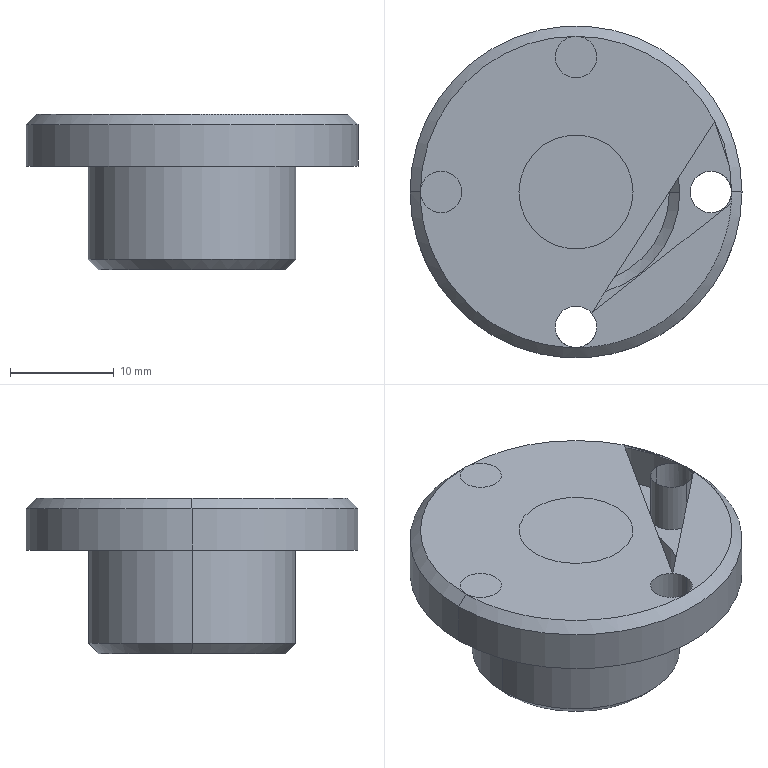Part | SolidWorks | features ICE 3, Chamfer 1, CirPattern 1, Extrusion 1 | 1 solid | 21 faces | box 32 x 32 x 15 mm | volume 5406 mm3 | cylinder 14 | cone 4 | plane 3 | commonest cylinder face diameters 4 x8 11 x2 20 x2 32 x2
STEP:
#1=CARTESIAN_POINT('',(-5.5,0.,15.));
#2=VERTEX_POINT('',#1);
#3=CARTESIAN_POINT('',(5.5,0.,15.));
#4=VERTEX_POINT('',#3);
#5=CARTESIAN_POINT('',(0.,0.,15.));
#6=DIRECTION('',(0.,0.,1.));
#7=DIRECTION('',(1.,0.,0.));
#8=AXIS2_PLACEMENT_3D('',#5,#6,#7);
#9=CIRCLE('',#8,5.5);
#10=EDGE_CURVE('',#2,#4,#9,.T.);
#11=ORIENTED_EDGE('',*,*,#10,.T.);
#12=CARTESIAN_POINT('',(5.5,0.,0.));
#13=VERTEX_POINT('',#12);
#14=CARTESIAN_POINT('',(5.5,0.,29.));
#15=DIRECTION('',(0.,0.,-1.));
#16=VECTOR('',#15,1000.);
#17=LINE('',#14,#16);
#18=EDGE_CURVE('',#4,#13,#17,.T.);
#19=ORIENTED_EDGE('',*,*,#18,.T.);
#20=CARTESIAN_POINT('',(-5.5,0.,0.));
#21=VERTEX_POINT('',#20);
#22=CARTESIAN_POINT('',(0.,0.,0.));
#23=DIRECTION('',(0.,0.,-1.));
#24=DIRECTION('',(-1.,0.,0.));
#25=AXIS2_PLACEMENT_3D('',#22,#23,#24);
#26=CIRCLE('',#25,5.5);
#27=EDGE_CURVE('',#13,#21,#26,.T.);
#28=ORIENTED_EDGE('',*,*,#27,.T.);
#29=CARTESIAN_POINT('',(-5.5,0.,29.));
#30=DIRECTION('',(0.,0.,-1.));
#31=VECTOR('',#30,1000.);
#32=LINE('',#29,#31);
#33=EDGE_CURVE('',#2,#21,#32,.T.);
#34=ORIENTED_EDGE('',*,*,#33,.F.);
#35=EDGE_LOOP('',(#11,#19,#28,#34));
#36=FACE_OUTER_BOUND('',#35,.T.);
#37=CARTESIAN_POINT('',(0.,0.,29.));
#38=DIRECTION('',(0.,0.,-1.));
#39=DIRECTION('',(-1.,0.,0.));
#40=AXIS2_PLACEMENT_3D('',#37,#38,#39);
#41=CYLINDRICAL_SURFACE('',#40,5.5);
#42=ADVANCED_FACE('',(#36),#41,.F.);
#43=CARTESIAN_POINT('',(-13.,-2.,15.));
#44=VERTEX_POINT('',#43);
#45=CARTESIAN_POINT('',(-13.,2.,15.));
#46=VERTEX_POINT('',#45);
#47=CARTESIAN_POINT('',(-13.,0.,15.));
#48=DIRECTION('',(0.,0.,1.));
#49=DIRECTION('',(0.,1.,0.));
#50=AXIS2_PLACEMENT_3D('',#47,#48,#49);
#51=CIRCLE('',#50,2.);
#52=EDGE_CURVE('',#44,#46,#51,.T.);
#53=ORIENTED_EDGE('',*,*,#52,.T.);
#54=CARTESIAN_POINT('',(-13.,2.,10.));
#55=VERTEX_POINT('',#54);
#56=CARTESIAN_POINT('',(-13.,2.,20.));
#57=DIRECTION('',(0.,0.,-1.));
#58=VECTOR('',#57,1000.);
#59=LINE('',#56,#58);
#60=EDGE_CURVE('',#46,#55,#59,.T.);
#61=ORIENTED_EDGE('',*,*,#60,.T.);
#62=CARTESIAN_POINT('',(-13.,-2.,10.));
#63=VERTEX_POINT('',#62);
#64=CARTESIAN_POINT('',(-13.,0.,10.));
#65=DIRECTION('',(0.,0.,-1.));
#66=DIRECTION('',(0.,-1.,0.));
#67=AXIS2_PLACEMENT_3D('',#64,#65,#66);
#68=CIRCLE('',#67,2.);
#69=EDGE_CURVE('',#55,#63,#68,.T.);
#70=ORIENTED_EDGE('',*,*,#69,.T.);
#71=CARTESIAN_POINT('',(-13.,-2.,20.));
#72=DIRECTION('',(0.,0.,-1.));
#73=VECTOR('',#72,1000.);
#74=LINE('',#71,#73);
#75=EDGE_CURVE('',#44,#63,#74,.T.);
#76=ORIENTED_EDGE('',*,*,#75,.F.);
#77=EDGE_LOOP('',(#53,#61,#70,#76));
#78=FACE_OUTER_BOUND('',#77,.T.);
#79=CARTESIAN_POINT('',(-13.,0.,20.));
#80=DIRECTION('',(0.,0.,-1.));
#81=DIRECTION('',(0.,-1.,0.));
#82=AXIS2_PLACEMENT_3D('',#79,#80,#81);
#83=CYLINDRICAL_SURFACE('',#82,2.);
#84=ADVANCED_FACE('',(#78),#83,.F.);
#85=CARTESIAN_POINT('',(2.,-13.,15.));
#86=VERTEX_POINT('',#85);
#87=CARTESIAN_POINT('',(-2.,-13.,15.));
#88=VERTEX_POINT('',#87);
#89=CARTESIAN_POINT('',(0.,-13.,15.));
#90=DIRECTION('',(0.,0.,1.));
#91=DIRECTION('',(-1.,0.,0.));
#92=AXIS2_PLACEMENT_3D('',#89,#90,#91);
#93=CIRCLE('',#92,2.);
#94=EDGE_CURVE('',#86,#88,#93,.T.);
#95=ORIENTED_EDGE('',*,*,#94,.T.);
#96=CARTESIAN_POINT('',(-2.,-13.,10.));
#97=VERTEX_POINT('',#96);
#98=CARTESIAN_POINT('',(-2.,-13.,20.));
#99=DIRECTION('',(0.,0.,-1.));
#100=VECTOR('',#99,1000.);
#101=LINE('',#98,#100);
#102=EDGE_CURVE('',#88,#97,#101,.T.);
#103=ORIENTED_EDGE('',*,*,#102,.T.);
#104=CARTESIAN_POINT('',(2.,-13.,10.));
#105=VERTEX_POINT('',#104);
#106=CARTESIAN_POINT('',(0.,-13.,10.));
#107=DIRECTION('',(0.,0.,-1.));
#108=DIRECTION('',(1.,0.,0.));
#109=AXIS2_PLACEMENT_3D('',#106,#107,#108);
#110=CIRCLE('',#109,2.);
#111=EDGE_CURVE('',#97,#105,#110,.T.);
#112=ORIENTED_EDGE('',*,*,#111,.T.);
#113=CARTESIAN_POINT('',(2.,-13.,20.));
#114=DIRECTION('',(0.,0.,-1.));
#115=VECTOR('',#114,1000.);
#116=LINE('',#113,#115);
#117=EDGE_CURVE('',#86,#105,#116,.T.);
#118=ORIENTED_EDGE('',*,*,#117,.F.);
#119=EDGE_LOOP('',(#95,#103,#112,#118));
#120=FACE_OUTER_BOUND('',#119,.T.);
#121=CARTESIAN_POINT('',(0.,-13.,20.));
#122=DIRECTION('',(0.,0.,-1.));
#123=DIRECTION('',(1.,0.,0.));
#124=AXIS2_PLACEMENT_3D('',#121,#122,#123);
#125=CYLINDRICAL_SURFACE('',#124,2.);
#126=ADVANCED_FACE('',(#120),#125,.F.);
#127=CARTESIAN_POINT('',(13.,2.,15.));
#128=VERTEX_POINT('',#127);
#129=CARTESIAN_POINT('',(13.,-2.,15.));
#130=VERTEX_POINT('',#129);
#131=CARTESIAN_POINT('',(13.,0.,15.));
#132=DIRECTION('',(0.,0.,1.));
#133=DIRECTION('',(0.,-1.,0.));
#134=AXIS2_PLACEMENT_3D('',#131,#132,#133);
#135=CIRCLE('',#134,2.);
#136=EDGE_CURVE('',#128,#130,#135,.T.);
#137=ORIENTED_EDGE('',*,*,#136,.T.);
#138=CARTESIAN_POINT('',(13.,-2.,10.));
#139=VERTEX_POINT('',#138);
#140=CARTESIAN_POINT('',(13.,-2.,20.));
#141=DIRECTION('',(0.,0.,-1.));
#142=VECTOR('',#141,1000.);
#143=LINE('',#140,#142);
#144=EDGE_CURVE('',#130,#139,#143,.T.);
#145=ORIENTED_EDGE('',*,*,#144,.T.);
#146=CARTESIAN_POINT('',(13.,2.,10.));
#147=VERTEX_POINT('',#146);
#148=CARTESIAN_POINT('',(13.,0.,10.));
#149=DIRECTION('',(0.,0.,-1.));
#150=DIRECTION('',(0.,1.,0.));
#151=AXIS2_PLACEMENT_3D('',#148,#149,#150);
#152=CIRCLE('',#151,2.);
#153=EDGE_CURVE('',#139,#147,#152,.T.);
#154=ORIENTED_EDGE('',*,*,#153,.T.);
#155=CARTESIAN_POINT('',(13.,2.,20.));
#156=DIRECTION('',(0.,0.,-1.));
#157=VECTOR('',#156,1000.);
#158=LINE('',#155,#157);
#159=EDGE_CURVE('',#128,#147,#158,.T.);
#160=ORIENTED_EDGE('',*,*,#159,.F.);
#161=EDGE_LOOP('',(#137,#145,#154,#160));
#162=FACE_OUTER_BOUND('',#161,.T.);
#163=CARTESIAN_POINT('',(13.,0.,20.));
#164=DIRECTION('',(0.,0.,-1.));
#165=DIRECTION('',(0.,1.,0.));
#166=AXIS2_PLACEMENT_3D('',#163,#164,#165);
#167=CYLINDRICAL_SURFACE('',#166,2.);
#168=ADVANCED_FACE('',(#162),#167,.F.);
#169=CARTESIAN_POINT('',(-2.,13.,15.));
#170=VERTEX_POINT('',#169);
#171=CARTESIAN_POINT('',(2.,13.,15.));
#172=VERTEX_POINT('',#171);
#173=CARTESIAN_POINT('',(0.,13.,15.));
#174=DIRECTION('',(0.,0.,1.));
#175=DIRECTION('',(1.,0.,0.));
#176=AXIS2_PLACEMENT_3D('',#173,#174,#175);
#177=CIRCLE('',#176,2.);
#178=EDGE_CURVE('',#170,#172,#177,.T.);
#179=ORIENTED_EDGE('',*,*,#178,.T.);
#180=CARTESIAN_POINT('',(2.,13.,10.));
#181=VERTEX_POINT('',#180);
#182=CARTESIAN_POINT('',(2.,13.,20.));
#183=DIRECTION('',(0.,0.,-1.));
#184=VECTOR('',#183,1000.);
#185=LINE('',#182,#184);
#186=EDGE_CURVE('',#172,#181,#185,.T.);
#187=ORIENTED_EDGE('',*,*,#186,.T.);
#188=CARTESIAN_POINT('',(-2.,13.,10.));
#189=VERTEX_POINT('',#188);
#190=CARTESIAN_POINT('',(0.,13.,10.));
#191=DIRECTION('',(0.,0.,-1.));
#192=DIRECTION('',(-1.,0.,0.));
#193=AXIS2_PLACEMENT_3D('',#190,#191,#192);
#194=CIRCLE('',#193,2.);
#195=EDGE_CURVE('',#181,#189,#194,.T.);
#196=ORIENTED_EDGE('',*,*,#195,.T.);
#197=CARTESIAN_POINT('',(-2.,13.,20.));
#198=DIRECTION('',(0.,0.,-1.));
#199=VECTOR('',#198,1000.);
#200=LINE('',#197,#199);
#201=EDGE_CURVE('',#170,#189,#200,.T.);
#202=ORIENTED_EDGE('',*,*,#201,.F.);
#203=EDGE_LOOP('',(#179,#187,#196,#202));
#204=FACE_OUTER_BOUND('',#203,.T.);
#205=CARTESIAN_POINT('',(0.,13.,20.));
#206=DIRECTION('',(0.,0.,-1.));
#207=DIRECTION('',(-1.,0.,0.));
#208=AXIS2_PLACEMENT_3D('',#205,#206,#207);
#209=CYLINDRICAL_SURFACE('',#208,2.);
#210=ADVANCED_FACE('',(#204),#209,.F.);
#211=CARTESIAN_POINT('',(15.,0.,15.));
#212=VERTEX_POINT('',#211);
#213=CARTESIAN_POINT('',(0.,15.,15.));
#214=VERTEX_POINT('',#213);
#215=CARTESIAN_POINT('',(0.,0.,15.));
#216=DIRECTION('',(0.,0.,1.));
#217=DIRECTION('',(1.,0.,0.));
#218=AXIS2_PLACEMENT_3D('',#215,#216,#217);
#219=CIRCLE('',#218,15.);
#220=EDGE_CURVE('',#212,#214,#219,.T.);
#221=ORIENTED_EDGE('',*,*,#220,.F.);
#222=CARTESIAN_POINT('',(16.,0.,14.));
#223=VERTEX_POINT('',#222);
#224=CARTESIAN_POINT('',(15.,0.,15.));
#225=DIRECTION('',(0.7071,0.,-0.7071));
#226=VECTOR('',#225,1000.);
#227=LINE('',#224,#226);
#228=EDGE_CURVE('',#212,#223,#227,.T.);
#229=ORIENTED_EDGE('',*,*,#228,.T.);
#230=CARTESIAN_POINT('',(-16.,0.,14.));
#231=VERTEX_POINT('',#230);
#232=CARTESIAN_POINT('',(0.,0.,14.));
#233=DIRECTION('',(0.,0.,-1.));
#234=DIRECTION('',(1.,0.,0.));
#235=AXIS2_PLACEMENT_3D('',#232,#233,#234);
#236=CIRCLE('',#235,16.);
#237=EDGE_CURVE('',#231,#223,#236,.T.);
#238=ORIENTED_EDGE('',*,*,#237,.F.);
#239=CARTESIAN_POINT('',(-15.,0.,15.));
#240=VERTEX_POINT('',#239);
#241=CARTESIAN_POINT('',(-15.,0.,15.));
#242=DIRECTION('',(-0.7071,0.,-0.7071));
#243=VECTOR('',#242,1000.);
#244=LINE('',#241,#243);
#245=EDGE_CURVE('',#240,#231,#244,.T.);
#246=ORIENTED_EDGE('',*,*,#245,.F.);
#247=CARTESIAN_POINT('',(0.,0.,15.));
#248=DIRECTION('',(0.,0.,1.));
#249=DIRECTION('',(1.,0.,0.));
#250=AXIS2_PLACEMENT_3D('',#247,#248,#249);
#251=CIRCLE('',#250,15.);
#252=EDGE_CURVE('',#214,#240,#251,.T.);
#253=ORIENTED_EDGE('',*,*,#252,.F.);
#254=EDGE_LOOP('',(#221,#229,#238,#246,#253));
#255=FACE_OUTER_BOUND('',#254,.T.);
#256=CARTESIAN_POINT('',(0.,0.,15.));
#257=DIRECTION('',(0.,0.,-1.));
#258=DIRECTION('',(-1.,0.,0.));
#259=AXIS2_PLACEMENT_3D('',#256,#257,#258);
#260=CONICAL_SURFACE('',#259,15.,0.7854);
#261=ADVANCED_FACE('',(#255),#260,.T.);
#262=CARTESIAN_POINT('',(-9.,0.,0.));
#263=VERTEX_POINT('',#262);
#264=CARTESIAN_POINT('',(9.,0.,0.));
#265=VERTEX_POINT('',#264);
#266=CARTESIAN_POINT('',(0.,0.,0.));
#267=DIRECTION('',(0.,0.,-1.));
#268=DIRECTION('',(1.,0.,0.));
#269=AXIS2_PLACEMENT_3D('',#266,#267,#268);
#270=CIRCLE('',#269,9.);
#271=EDGE_CURVE('',#263,#265,#270,.T.);
#272=ORIENTED_EDGE('',*,*,#271,.F.);
#273=CARTESIAN_POINT('',(-10.,0.,1.));
#274=VERTEX_POINT('',#273);
#275=CARTESIAN_POINT('',(-10.,0.,1.));
#276=DIRECTION('',(-0.7071,0.,0.7071));
#277=VECTOR('',#276,1000.);
#278=LINE('',#275,#277);
#279=EDGE_CURVE('',#263,#274,#278,.T.);
#280=ORIENTED_EDGE('',*,*,#279,.T.);
#281=CARTESIAN_POINT('',(10.,0.,1.));
#282=VERTEX_POINT('',#281);
#283=CARTESIAN_POINT('',(0.,0.,1.));
#284=DIRECTION('',(0.,0.,1.));
#285=DIRECTION('',(1.,0.,0.));
#286=AXIS2_PLACEMENT_3D('',#283,#284,#285);
#287=CIRCLE('',#286,10.);
#288=EDGE_CURVE('',#282,#274,#287,.T.);
#289=ORIENTED_EDGE('',*,*,#288,.F.);
#290=CARTESIAN_POINT('',(10.,0.,1.));
#291=DIRECTION('',(0.7071,0.,0.7071));
#292=VECTOR('',#291,1000.);
#293=LINE('',#290,#292);
#294=EDGE_CURVE('',#265,#282,#293,.T.);
#295=ORIENTED_EDGE('',*,*,#294,.F.);
#296=EDGE_LOOP('',(#272,#280,#289,#295));
#297=FACE_OUTER_BOUND('',#296,.T.);
#298=CARTESIAN_POINT('',(0.,0.,1.));
#299=DIRECTION('',(0.,0.,1.));
#300=DIRECTION('',(1.,0.,0.));
#301=AXIS2_PLACEMENT_3D('',#298,#299,#300);
#302=CONICAL_SURFACE('',#301,10.,0.7854);
#303=ADVANCED_FACE('',(#297),#302,.T.);
#304=ORIENTED_EDGE('',*,*,#237,.T.);
#305=CARTESIAN_POINT('',(16.,0.,10.));
#306=VERTEX_POINT('',#305);
#307=CARTESIAN_POINT('',(16.,0.,15.));
#308=DIRECTION('',(0.,0.,-1.));
#309=VECTOR('',#308,1000.);
#310=LINE('',#307,#309);
#311=EDGE_CURVE('',#223,#306,#310,.T.);
#312=ORIENTED_EDGE('',*,*,#311,.T.);
#313=CARTESIAN_POINT('',(-16.,0.,10.));
#314=VERTEX_POINT('',#313);
#315=CARTESIAN_POINT('',(0.,0.,10.));
#316=DIRECTION('',(0.,0.,1.));
#317=DIRECTION('',(1.,0.,0.));
#318=AXIS2_PLACEMENT_3D('',#315,#316,#317);
#319=CIRCLE('',#318,16.);
#320=EDGE_CURVE('',#306,#314,#319,.T.);
#321=ORIENTED_EDGE('',*,*,#320,.T.);
#322=CARTESIAN_POINT('',(-16.,0.,15.));
#323=DIRECTION('',(0.,0.,-1.));
#324=VECTOR('',#323,1000.);
#325=LINE('',#322,#324);
#326=EDGE_CURVE('',#231,#314,#325,.T.);
#327=ORIENTED_EDGE('',*,*,#326,.F.);
#328=EDGE_LOOP('',(#304,#312,#321,#327));
#329=FACE_OUTER_BOUND('',#328,.T.);
#330=CARTESIAN_POINT('',(0.,0.,15.));
#331=DIRECTION('',(0.,0.,-1.));
#332=DIRECTION('',(-1.,0.,0.));
#333=AXIS2_PLACEMENT_3D('',#330,#331,#332);
#334=CYLINDRICAL_SURFACE('',#333,16.);
#335=ADVANCED_FACE('',(#329),#334,.T.);
#336=CARTESIAN_POINT('',(10.,0.,10.));
#337=VERTEX_POINT('',#336);
#338=CARTESIAN_POINT('',(-10.,0.,10.));
#339=VERTEX_POINT('',#338);
#340=CARTESIAN_POINT('',(0.,0.,10.));
#341=DIRECTION('',(0.,0.,1.));
#342=DIRECTION('',(1.,0.,0.));
#343=AXIS2_PLACEMENT_3D('',#340,#341,#342);
#344=CIRCLE('',#343,10.);
#345=EDGE_CURVE('',#337,#339,#344,.T.);
#346=ORIENTED_EDGE('',*,*,#345,.F.);
#347=CARTESIAN_POINT('',(10.,0.,10.));
#348=DIRECTION('',(0.,0.,-1.));
#349=VECTOR('',#348,1000.);
#350=LINE('',#347,#349);
#351=EDGE_CURVE('',#337,#282,#350,.T.);
#352=ORIENTED_EDGE('',*,*,#351,.T.);
#353=ORIENTED_EDGE('',*,*,#288,.T.);
#354=CARTESIAN_POINT('',(-10.,0.,10.));
#355=DIRECTION('',(0.,0.,-1.));
#356=VECTOR('',#355,1000.);
#357=LINE('',#354,#356);
#358=EDGE_CURVE('',#339,#274,#357,.T.);
#359=ORIENTED_EDGE('',*,*,#358,.F.);
#360=EDGE_LOOP('',(#346,#352,#353,#359));
#361=FACE_OUTER_BOUND('',#360,.T.);
#362=CARTESIAN_POINT('',(0.,0.,10.));
#363=DIRECTION('',(0.,0.,-1.));
#364=DIRECTION('',(-1.,0.,0.));
#365=AXIS2_PLACEMENT_3D('',#362,#363,#364);
#366=CYLINDRICAL_SURFACE('',#365,10.);
#367=ADVANCED_FACE('',(#361),#366,.T.);
#368=ORIENTED_EDGE('',*,*,#351,.F.);
#369=CARTESIAN_POINT('',(0.,0.,10.));
#370=DIRECTION('',(0.,0.,1.));
#371=DIRECTION('',(1.,0.,0.));
#372=AXIS2_PLACEMENT_3D('',#369,#370,#371);
#373=CIRCLE('',#372,10.);
#374=EDGE_CURVE('',#339,#337,#373,.T.);
#375=ORIENTED_EDGE('',*,*,#374,.F.);
#376=ORIENTED_EDGE('',*,*,#358,.T.);
#377=CARTESIAN_POINT('',(0.,0.,1.));
#378=DIRECTION('',(0.,0.,1.));
#379=DIRECTION('',(1.,0.,0.));
#380=AXIS2_PLACEMENT_3D('',#377,#378,#379);
#381=CIRCLE('',#380,10.);
#382=EDGE_CURVE('',#274,#282,#381,.T.);
#383=ORIENTED_EDGE('',*,*,#382,.T.);
#384=EDGE_LOOP('',(#368,#375,#376,#383));
#385=FACE_OUTER_BOUND('',#384,.T.);
#386=CARTESIAN_POINT('',(0.,0.,10.));
#387=DIRECTION('',(0.,0.,-1.));
#388=DIRECTION('',(-1.,0.,0.));
#389=AXIS2_PLACEMENT_3D('',#386,#387,#388);
#390=CYLINDRICAL_SURFACE('',#389,10.);
#391=ADVANCED_FACE('',(#385),#390,.T.);
#392=CARTESIAN_POINT('',(0.,0.,0.));
#393=DIRECTION('',(0.,0.,-1.));
#394=DIRECTION('',(-1.,0.,0.));
#395=AXIS2_PLACEMENT_3D('',#392,#393,#394);
#396=CIRCLE('',#395,5.5);
#397=EDGE_CURVE('',#21,#13,#396,.T.);
#398=ORIENTED_EDGE('',*,*,#397,.F.);
#399=ORIENTED_EDGE('',*,*,#27,.F.);
#400=EDGE_LOOP('',(#398,#399));
#401=FACE_BOUND('',#400,.T.);
#402=CARTESIAN_POINT('',(0.,0.,0.));
#403=DIRECTION('',(0.,0.,-1.));
#404=DIRECTION('',(1.,0.,0.));
#405=AXIS2_PLACEMENT_3D('',#402,#403,#404);
#406=CIRCLE('',#405,9.);
#407=EDGE_CURVE('',#265,#263,#406,.T.);
#408=ORIENTED_EDGE('',*,*,#407,.T.);
#409=ORIENTED_EDGE('',*,*,#271,.T.);
#410=EDGE_LOOP('',(#408,#409));
#411=FACE_OUTER_BOUND('',#410,.T.);
#412=CARTESIAN_POINT('',(0.,0.,0.));
#413=DIRECTION('',(0.,0.,1.));
#414=DIRECTION('',(1.,0.,0.));
#415=AXIS2_PLACEMENT_3D('',#412,#413,#414);
#416=PLANE('',#415);
#417=ADVANCED_FACE('',(#401,#411),#416,.F.);
#418=CARTESIAN_POINT('',(-13.,0.,10.));
#419=DIRECTION('',(0.,0.,-1.));
#420=DIRECTION('',(0.,-1.,0.));
#421=AXIS2_PLACEMENT_3D('',#418,#419,#420);
#422=CIRCLE('',#421,2.);
#423=EDGE_CURVE('',#63,#55,#422,.T.);
#424=ORIENTED_EDGE('',*,*,#423,.F.);
#425=ORIENTED_EDGE('',*,*,#69,.F.);
#426=EDGE_LOOP('',(#424,#425));
#427=FACE_BOUND('',#426,.T.);
#428=CARTESIAN_POINT('',(0.,-13.,10.));
#429=DIRECTION('',(0.,0.,-1.));
#430=DIRECTION('',(1.,0.,0.));
#431=AXIS2_PLACEMENT_3D('',#428,#429,#430);
#432=CIRCLE('',#431,2.);
#433=EDGE_CURVE('',#105,#97,#432,.T.);
#434=ORIENTED_EDGE('',*,*,#433,.F.);
#435=ORIENTED_EDGE('',*,*,#111,.F.);
#436=EDGE_LOOP('',(#434,#435));
#437=FACE_BOUND('',#436,.T.);
#438=CARTESIAN_POINT('',(13.,0.,10.));
#439=DIRECTION('',(0.,0.,-1.));
#440=DIRECTION('',(0.,1.,0.));
#441=AXIS2_PLACEMENT_3D('',#438,#439,#440);
#442=CIRCLE('',#441,2.);
#443=EDGE_CURVE('',#147,#139,#442,.T.);
#444=ORIENTED_EDGE('',*,*,#443,.F.);
#445=ORIENTED_EDGE('',*,*,#153,.F.);
#446=EDGE_LOOP('',(#444,#445));
#447=FACE_BOUND('',#446,.T.);
#448=CARTESIAN_POINT('',(0.,13.,10.));
#449=DIRECTION('',(0.,0.,-1.));
#450=DIRECTION('',(-1.,0.,0.));
#451=AXIS2_PLACEMENT_3D('',#448,#449,#450);
#452=CIRCLE('',#451,2.);
#453=EDGE_CURVE('',#189,#181,#452,.T.);
#454=ORIENTED_EDGE('',*,*,#453,.F.);
#455=ORIENTED_EDGE('',*,*,#195,.F.);
#456=EDGE_LOOP('',(#454,#455));
#457=FACE_BOUND('',#456,.T.);
#458=CARTESIAN_POINT('',(0.,0.,10.));
#459=DIRECTION('',(0.,0.,1.));
#460=DIRECTION('',(1.,0.,0.));
#461=AXIS2_PLACEMENT_3D('',#458,#459,#460);
#462=CIRCLE('',#461,16.);
#463=EDGE_CURVE('',#314,#306,#462,.T.);
#464=ORIENTED_EDGE('',*,*,#463,.F.);
#465=ORIENTED_EDGE('',*,*,#320,.F.);
#466=EDGE_LOOP('',(#464,#465));
#467=FACE_OUTER_BOUND('',#466,.T.);
#468=ORIENTED_EDGE('',*,*,#374,.T.);
#469=ORIENTED_EDGE('',*,*,#345,.T.);
#470=EDGE_LOOP('',(#468,#469));
#471=FACE_BOUND('',#470,.T.);
#472=CARTESIAN_POINT('',(0.,0.,10.));
#473=DIRECTION('',(0.,0.,1.));
#474=DIRECTION('',(1.,0.,0.));
#475=AXIS2_PLACEMENT_3D('',#472,#473,#474);
#476=PLANE('',#475);
#477=ADVANCED_FACE('',(#427,#437,#447,#457,#467,#471),#476,.F.);
#478=ORIENTED_EDGE('',*,*,#311,.F.);
#479=CARTESIAN_POINT('',(0.,0.,14.));
#480=DIRECTION('',(0.,0.,-1.));
#481=DIRECTION('',(1.,0.,0.));
#482=AXIS2_PLACEMENT_3D('',#479,#480,#481);
#483=CIRCLE('',#482,16.);
#484=EDGE_CURVE('',#223,#231,#483,.T.);
#485=ORIENTED_EDGE('',*,*,#484,.T.);
#486=ORIENTED_EDGE('',*,*,#326,.T.);
#487=ORIENTED_EDGE('',*,*,#463,.T.);
#488=EDGE_LOOP('',(#478,#485,#486,#487));
#489=FACE_OUTER_BOUND('',#488,.T.);
#490=CARTESIAN_POINT('',(0.,0.,15.));
#491=DIRECTION('',(0.,0.,-1.));
#492=DIRECTION('',(-1.,0.,0.));
#493=AXIS2_PLACEMENT_3D('',#490,#491,#492);
#494=CYLINDRICAL_SURFACE('',#493,16.);
#495=ADVANCED_FACE('',(#489),#494,.T.);
#496=ORIENTED_EDGE('',*,*,#10,.F.);
#497=CARTESIAN_POINT('',(0.,0.,15.));
#498=DIRECTION('',(0.,0.,1.));
#499=DIRECTION('',(1.,0.,0.));
#500=AXIS2_PLACEMENT_3D('',#497,#498,#499);
#501=CIRCLE('',#500,5.5);
#502=EDGE_CURVE('',#4,#2,#501,.T.);
#503=ORIENTED_EDGE('',*,*,#502,.F.);
#504=EDGE_LOOP('',(#496,#503));
#505=FACE_BOUND('',#504,.T.);
#506=ORIENTED_EDGE('',*,*,#252,.T.);
#507=CARTESIAN_POINT('',(-13.,0.,15.));
#508=DIRECTION('',(0.,0.,1.));
#509=DIRECTION('',(0.,1.,0.));
#510=AXIS2_PLACEMENT_3D('',#507,#508,#509);
#511=CIRCLE('',#510,2.);
#512=EDGE_CURVE('',#46,#240,#511,.T.);
#513=ORIENTED_EDGE('',*,*,#512,.F.);
#514=ORIENTED_EDGE('',*,*,#52,.F.);
#515=CARTESIAN_POINT('',(-13.,0.,15.));
#516=DIRECTION('',(0.,0.,1.));
#517=DIRECTION('',(0.,1.,0.));
#518=AXIS2_PLACEMENT_3D('',#515,#516,#517);
#519=CIRCLE('',#518,2.);
#520=EDGE_CURVE('',#240,#44,#519,.T.);
#521=ORIENTED_EDGE('',*,*,#520,.F.);
#522=CARTESIAN_POINT('',(0.,-15.,15.));
#523=VERTEX_POINT('',#522);
#524=CARTESIAN_POINT('',(0.,0.,15.));
#525=DIRECTION('',(0.,0.,1.));
#526=DIRECTION('',(1.,0.,0.));
#527=AXIS2_PLACEMENT_3D('',#524,#525,#526);
#528=CIRCLE('',#527,15.);
#529=EDGE_CURVE('',#240,#523,#528,.T.);
#530=ORIENTED_EDGE('',*,*,#529,.T.);
#531=CARTESIAN_POINT('',(0.,-13.,15.));
#532=DIRECTION('',(0.,0.,1.));
#533=DIRECTION('',(-1.,0.,0.));
#534=AXIS2_PLACEMENT_3D('',#531,#532,#533);
#535=CIRCLE('',#534,2.);
#536=EDGE_CURVE('',#88,#523,#535,.T.);
#537=ORIENTED_EDGE('',*,*,#536,.F.);
#538=ORIENTED_EDGE('',*,*,#94,.F.);
#539=CARTESIAN_POINT('',(0.,-13.,15.));
#540=DIRECTION('',(0.,0.,1.));
#541=DIRECTION('',(-1.,0.,0.));
#542=AXIS2_PLACEMENT_3D('',#539,#540,#541);
#543=CIRCLE('',#542,2.);
#544=EDGE_CURVE('',#523,#86,#543,.T.);
#545=ORIENTED_EDGE('',*,*,#544,.F.);
#546=CARTESIAN_POINT('',(0.,0.,15.));
#547=DIRECTION('',(0.,0.,1.));
#548=DIRECTION('',(1.,0.,0.));
#549=AXIS2_PLACEMENT_3D('',#546,#547,#548);
#550=CIRCLE('',#549,15.);
#551=EDGE_CURVE('',#523,#212,#550,.T.);
#552=ORIENTED_EDGE('',*,*,#551,.T.);
#553=CARTESIAN_POINT('',(13.,0.,15.));
#554=DIRECTION('',(0.,0.,1.));
#555=DIRECTION('',(0.,-1.,0.));
#556=AXIS2_PLACEMENT_3D('',#553,#554,#555);
#557=CIRCLE('',#556,2.);
#558=EDGE_CURVE('',#130,#212,#557,.T.);
#559=ORIENTED_EDGE('',*,*,#558,.F.);
#560=ORIENTED_EDGE('',*,*,#136,.F.);
#561=CARTESIAN_POINT('',(13.,0.,15.));
#562=DIRECTION('',(0.,0.,1.));
#563=DIRECTION('',(0.,-1.,0.));
#564=AXIS2_PLACEMENT_3D('',#561,#562,#563);
#565=CIRCLE('',#564,2.);
#566=EDGE_CURVE('',#212,#128,#565,.T.);
#567=ORIENTED_EDGE('',*,*,#566,.F.);
#568=ORIENTED_EDGE('',*,*,#220,.T.);
#569=CARTESIAN_POINT('',(0.,13.,15.));
#570=DIRECTION('',(0.,0.,1.));
#571=DIRECTION('',(1.,0.,0.));
#572=AXIS2_PLACEMENT_3D('',#569,#570,#571);
#573=CIRCLE('',#572,2.);
#574=EDGE_CURVE('',#172,#214,#573,.T.);
#575=ORIENTED_EDGE('',*,*,#574,.F.);
#576=ORIENTED_EDGE('',*,*,#178,.F.);
#577=CARTESIAN_POINT('',(0.,13.,15.));
#578=DIRECTION('',(0.,0.,1.));
#579=DIRECTION('',(1.,0.,0.));
#580=AXIS2_PLACEMENT_3D('',#577,#578,#579);
#581=CIRCLE('',#580,2.);
#582=EDGE_CURVE('',#214,#170,#581,.T.);
#583=ORIENTED_EDGE('',*,*,#582,.F.);
#584=EDGE_LOOP('',(#506,#513,#514,#521,#530,#537,#538,#545,#552,#559,#560,#567,#568,#575,#576,#583));
#585=FACE_OUTER_BOUND('',#584,.T.);
#586=CARTESIAN_POINT('',(0.,0.,15.));
#587=DIRECTION('',(0.,0.,1.));
#588=DIRECTION('',(1.,0.,0.));
#589=AXIS2_PLACEMENT_3D('',#586,#587,#588);
#590=PLANE('',#589);
#591=ADVANCED_FACE('',(#505,#585),#590,.T.);
#592=ORIENTED_EDGE('',*,*,#279,.F.);
#593=ORIENTED_EDGE('',*,*,#407,.F.);
#594=ORIENTED_EDGE('',*,*,#294,.T.);
#595=ORIENTED_EDGE('',*,*,#382,.F.);
#596=EDGE_LOOP('',(#592,#593,#594,#595));
#597=FACE_OUTER_BOUND('',#596,.T.);
#598=CARTESIAN_POINT('',(0.,0.,1.));
#599=DIRECTION('',(0.,0.,1.));
#600=DIRECTION('',(1.,0.,0.));
#601=AXIS2_PLACEMENT_3D('',#598,#599,#600);
#602=CONICAL_SURFACE('',#601,10.,0.7854);
#603=ADVANCED_FACE('',(#597),#602,.T.);
#604=ORIENTED_EDGE('',*,*,#228,.F.);
#605=ORIENTED_EDGE('',*,*,#551,.F.);
#606=ORIENTED_EDGE('',*,*,#529,.F.);
#607=ORIENTED_EDGE('',*,*,#245,.T.);
#608=ORIENTED_EDGE('',*,*,#484,.F.);
#609=EDGE_LOOP('',(#604,#605,#606,#607,#608));
#610=FACE_OUTER_BOUND('',#609,.T.);
#611=CARTESIAN_POINT('',(0.,0.,15.));
#612=DIRECTION('',(0.,0.,-1.));
#613=DIRECTION('',(-1.,0.,0.));
#614=AXIS2_PLACEMENT_3D('',#611,#612,#613);
#615=CONICAL_SURFACE('',#614,15.,0.7854);
#616=ADVANCED_FACE('',(#610),#615,.T.);
#617=ORIENTED_EDGE('',*,*,#186,.F.);
#618=ORIENTED_EDGE('',*,*,#574,.T.);
#619=ORIENTED_EDGE('',*,*,#582,.T.);
#620=ORIENTED_EDGE('',*,*,#201,.T.);
#621=ORIENTED_EDGE('',*,*,#453,.T.);
#622=EDGE_LOOP('',(#617,#618,#619,#620,#621));
#623=FACE_OUTER_BOUND('',#622,.T.);
#624=CARTESIAN_POINT('',(0.,13.,20.));
#625=DIRECTION('',(0.,0.,-1.));
#626=DIRECTION('',(-1.,0.,0.));
#627=AXIS2_PLACEMENT_3D('',#624,#625,#626);
#628=CYLINDRICAL_SURFACE('',#627,2.);
#629=ADVANCED_FACE('',(#623),#628,.F.);
#630=ORIENTED_EDGE('',*,*,#144,.F.);
#631=ORIENTED_EDGE('',*,*,#558,.T.);
#632=ORIENTED_EDGE('',*,*,#566,.T.);
#633=ORIENTED_EDGE('',*,*,#159,.T.);
#634=ORIENTED_EDGE('',*,*,#443,.T.);
#635=EDGE_LOOP('',(#630,#631,#632,#633,#634));
#636=FACE_OUTER_BOUND('',#635,.T.);
#637=CARTESIAN_POINT('',(13.,0.,20.));
#638=DIRECTION('',(0.,0.,-1.));
#639=DIRECTION('',(0.,1.,0.));
#640=AXIS2_PLACEMENT_3D('',#637,#638,#639);
#641=CYLINDRICAL_SURFACE('',#640,2.);
#642=ADVANCED_FACE('',(#636),#641,.F.);
#643=ORIENTED_EDGE('',*,*,#102,.F.);
#644=ORIENTED_EDGE('',*,*,#536,.T.);
#645=ORIENTED_EDGE('',*,*,#544,.T.);
#646=ORIENTED_EDGE('',*,*,#117,.T.);
#647=ORIENTED_EDGE('',*,*,#433,.T.);
#648=EDGE_LOOP('',(#643,#644,#645,#646,#647));
#649=FACE_OUTER_BOUND('',#648,.T.);
#650=CARTESIAN_POINT('',(0.,-13.,20.));
#651=DIRECTION('',(0.,0.,-1.));
#652=DIRECTION('',(1.,0.,0.));
#653=AXIS2_PLACEMENT_3D('',#650,#651,#652);
#654=CYLINDRICAL_SURFACE('',#653,2.);
#655=ADVANCED_FACE('',(#649),#654,.F.);
#656=ORIENTED_EDGE('',*,*,#60,.F.);
#657=ORIENTED_EDGE('',*,*,#512,.T.);
#658=ORIENTED_EDGE('',*,*,#520,.T.);
#659=ORIENTED_EDGE('',*,*,#75,.T.);
#660=ORIENTED_EDGE('',*,*,#423,.T.);
#661=EDGE_LOOP('',(#656,#657,#658,#659,#660));
#662=FACE_OUTER_BOUND('',#661,.T.);
#663=CARTESIAN_POINT('',(-13.,0.,20.));
#664=DIRECTION('',(0.,0.,-1.));
#665=DIRECTION('',(0.,-1.,0.));
#666=AXIS2_PLACEMENT_3D('',#663,#664,#665);
#667=CYLINDRICAL_SURFACE('',#666,2.);
#668=ADVANCED_FACE('',(#662),#667,.F.);
#669=ORIENTED_EDGE('',*,*,#18,.F.);
#670=ORIENTED_EDGE('',*,*,#502,.T.);
#671=ORIENTED_EDGE('',*,*,#33,.T.);
#672=ORIENTED_EDGE('',*,*,#397,.T.);
#673=EDGE_LOOP('',(#669,#670,#671,#672));
#674=FACE_OUTER_BOUND('',#673,.T.);
#675=CARTESIAN_POINT('',(0.,0.,29.));
#676=DIRECTION('',(0.,0.,-1.));
#677=DIRECTION('',(-1.,0.,0.));
#678=AXIS2_PLACEMENT_3D('',#675,#676,#677);
#679=CYLINDRICAL_SURFACE('',#678,5.5);
#680=ADVANCED_FACE('',(#674),#679,.F.);
#681=CLOSED_SHELL('',(#42,#84,#126,#168,#210,#261,#303,#335,#367,#391,#417,#477,#495,#591,#603,#616,#629,#642,#655,#668,#680));
#682=MANIFOLD_SOLID_BREP('',#681);
#683=CARTESIAN_POINT('',(0.,0.,0.));
#684=DIRECTION('',(0.,0.,1.));
#685=DIRECTION('',(1.,0.,0.));
#686=AXIS2_PLACEMENT_3D('',#683,#684,#685);
#687=(LENGTH_UNIT()NAMED_UNIT(*)SI_UNIT(.MILLI.,.METRE.));
#688=UNCERTAINTY_MEASURE_WITH_UNIT(LENGTH_MEASURE(0.00001),#687,'','');
#689=(NAMED_UNIT(*)PLANE_ANGLE_UNIT()SI_UNIT($,.RADIAN.));
#690=(NAMED_UNIT(*)SI_UNIT($,.STERADIAN.)SOLID_ANGLE_UNIT());
#691=(GEOMETRIC_REPRESENTATION_CONTEXT(3)GLOBAL_UNCERTAINTY_ASSIGNED_CONTEXT((#688))GLOBAL_UNIT_ASSIGNED_CONTEXT((#687,#689,#690))REPRESENTATION_CONTEXT('',''));
#692=ADVANCED_BREP_SHAPE_REPRESENTATION('',(#682,#686),#691);